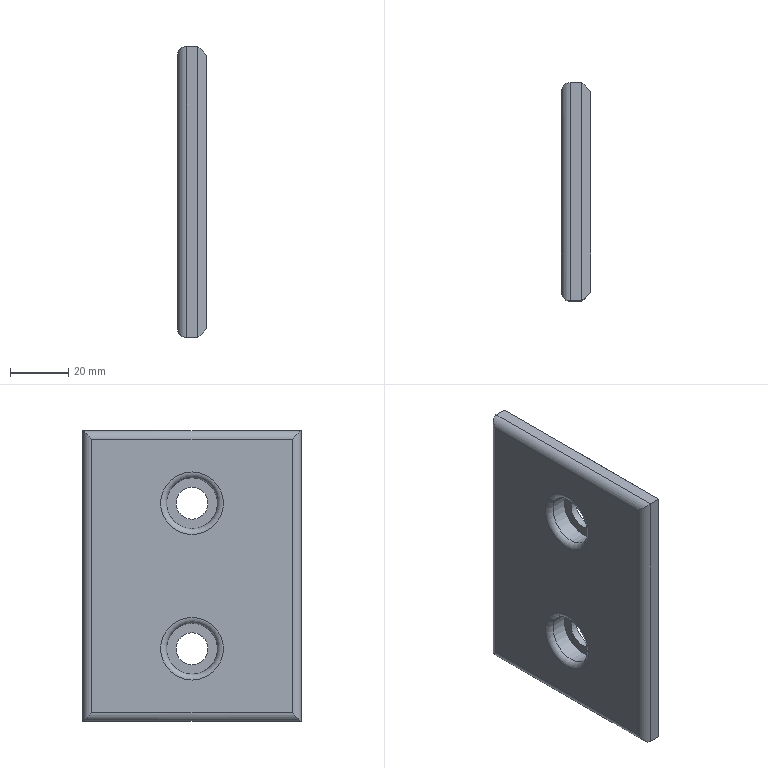Part | STEP file | lll_id4206_x_t | 1 solid | 157 faces | box 10 x 75 x 100 mm | volume 68604 mm3 | plane 112 | other 35 | cylinder 8 | torus 2 | commonest cylinder face diameters 6 x4 11 x2 17.5 x2